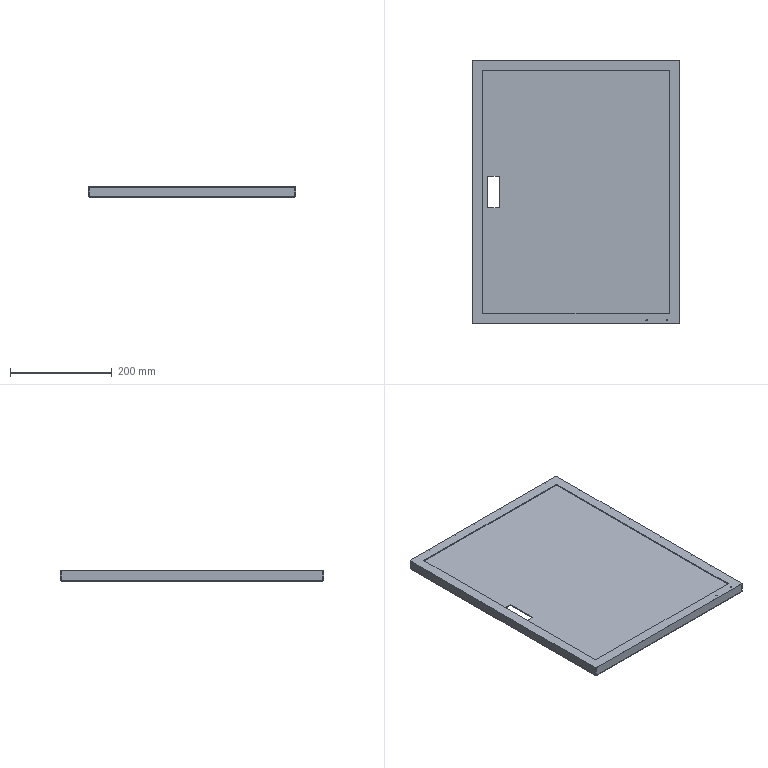Part | STEP file | 11-FG-JX00111 | 1 solid | 36 faces | box 408 x 519 x 20 mm | volume 549034 mm3 | plane 20 | cylinder 12 | sphere 4 | commonest cylinder face diameters 4 x8 2.5 x4
STEP:
#1=CARTESIAN_POINT('',(177.75,-252.5,18.));
#2=VERTEX_POINT('',#1);
#3=CARTESIAN_POINT('',(180.25,-252.5,18.));
#4=VERTEX_POINT('',#3);
#5=CARTESIAN_POINT('',(179.,-252.5,18.));
#6=DIRECTION('',(0.,0.,1.));
#7=DIRECTION('',(1.,0.,0.));
#8=AXIS2_PLACEMENT_3D('',#5,#6,#7);
#9=CIRCLE('',#8,1.25);
#10=EDGE_CURVE('',#2,#4,#9,.T.);
#11=ORIENTED_EDGE('',*,*,#10,.F.);
#12=CARTESIAN_POINT('',(177.75,-252.5,20.));
#13=VERTEX_POINT('',#12);
#14=CARTESIAN_POINT('',(177.75,-252.5,20.));
#15=DIRECTION('',(0.,0.,1.));
#16=VECTOR('',#15,1000.);
#17=LINE('',#14,#16);
#18=EDGE_CURVE('',#2,#13,#17,.T.);
#19=ORIENTED_EDGE('',*,*,#18,.T.);
#20=CARTESIAN_POINT('',(180.25,-252.5,20.));
#21=VERTEX_POINT('',#20);
#22=CARTESIAN_POINT('',(179.,-252.5,20.));
#23=DIRECTION('',(0.,0.,1.));
#24=DIRECTION('',(1.,0.,0.));
#25=AXIS2_PLACEMENT_3D('',#22,#23,#24);
#26=CIRCLE('',#25,1.25);
#27=EDGE_CURVE('',#13,#21,#26,.T.);
#28=ORIENTED_EDGE('',*,*,#27,.T.);
#29=CARTESIAN_POINT('',(180.25,-252.5,20.));
#30=DIRECTION('',(0.,0.,1.));
#31=VECTOR('',#30,1000.);
#32=LINE('',#29,#31);
#33=EDGE_CURVE('',#4,#21,#32,.T.);
#34=ORIENTED_EDGE('',*,*,#33,.F.);
#35=EDGE_LOOP('',(#11,#19,#28,#34));
#36=FACE_OUTER_BOUND('',#35,.T.);
#37=CARTESIAN_POINT('',(179.,-252.5,20.));
#38=DIRECTION('',(0.,0.,1.));
#39=DIRECTION('',(1.,0.,0.));
#40=AXIS2_PLACEMENT_3D('',#37,#38,#39);
#41=CYLINDRICAL_SURFACE('',#40,1.25);
#42=ADVANCED_FACE('',(#36),#41,.F.);
#43=CARTESIAN_POINT('',(137.75,-252.5,18.));
#44=VERTEX_POINT('',#43);
#45=CARTESIAN_POINT('',(140.25,-252.5,18.));
#46=VERTEX_POINT('',#45);
#47=CARTESIAN_POINT('',(139.,-252.5,18.));
#48=DIRECTION('',(0.,0.,1.));
#49=DIRECTION('',(1.,0.,0.));
#50=AXIS2_PLACEMENT_3D('',#47,#48,#49);
#51=CIRCLE('',#50,1.25);
#52=EDGE_CURVE('',#44,#46,#51,.T.);
#53=ORIENTED_EDGE('',*,*,#52,.F.);
#54=CARTESIAN_POINT('',(137.75,-252.5,20.));
#55=VERTEX_POINT('',#54);
#56=CARTESIAN_POINT('',(137.75,-252.5,20.));
#57=DIRECTION('',(0.,0.,1.));
#58=VECTOR('',#57,1000.);
#59=LINE('',#56,#58);
#60=EDGE_CURVE('',#44,#55,#59,.T.);
#61=ORIENTED_EDGE('',*,*,#60,.T.);
#62=CARTESIAN_POINT('',(140.25,-252.5,20.));
#63=VERTEX_POINT('',#62);
#64=CARTESIAN_POINT('',(139.,-252.5,20.));
#65=DIRECTION('',(0.,0.,1.));
#66=DIRECTION('',(1.,0.,0.));
#67=AXIS2_PLACEMENT_3D('',#64,#65,#66);
#68=CIRCLE('',#67,1.25);
#69=EDGE_CURVE('',#55,#63,#68,.T.);
#70=ORIENTED_EDGE('',*,*,#69,.T.);
#71=CARTESIAN_POINT('',(140.25,-252.5,20.));
#72=DIRECTION('',(0.,0.,1.));
#73=VECTOR('',#72,1000.);
#74=LINE('',#71,#73);
#75=EDGE_CURVE('',#46,#63,#74,.T.);
#76=ORIENTED_EDGE('',*,*,#75,.F.);
#77=EDGE_LOOP('',(#53,#61,#70,#76));
#78=FACE_OUTER_BOUND('',#77,.T.);
#79=CARTESIAN_POINT('',(139.,-252.5,20.));
#80=DIRECTION('',(0.,0.,1.));
#81=DIRECTION('',(1.,0.,0.));
#82=AXIS2_PLACEMENT_3D('',#79,#80,#81);
#83=CYLINDRICAL_SURFACE('',#82,1.25);
#84=ADVANCED_FACE('',(#78),#83,.F.);
#85=CARTESIAN_POINT('',(204.,-257.5,2.));
#86=VERTEX_POINT('',#85);
#87=CARTESIAN_POINT('',(204.,257.5,2.));
#88=VERTEX_POINT('',#87);
#89=CARTESIAN_POINT('',(204.,259.5,2.));
#90=DIRECTION('',(0.,1.,0.));
#91=VECTOR('',#90,1000.);
#92=LINE('',#89,#91);
#93=EDGE_CURVE('',#86,#88,#92,.T.);
#94=ORIENTED_EDGE('',*,*,#93,.T.);
#95=CARTESIAN_POINT('',(204.,257.5,20.));
#96=VERTEX_POINT('',#95);
#97=CARTESIAN_POINT('',(204.,257.5,20.));
#98=DIRECTION('',(0.,0.,1.));
#99=VECTOR('',#98,1000.);
#100=LINE('',#97,#99);
#101=EDGE_CURVE('',#88,#96,#100,.T.);
#102=ORIENTED_EDGE('',*,*,#101,.T.);
#103=CARTESIAN_POINT('',(204.,-257.5,20.));
#104=VERTEX_POINT('',#103);
#105=CARTESIAN_POINT('',(204.,259.5,20.));
#106=DIRECTION('',(0.,1.,0.));
#107=VECTOR('',#106,1000.);
#108=LINE('',#105,#107);
#109=EDGE_CURVE('',#104,#96,#108,.T.);
#110=ORIENTED_EDGE('',*,*,#109,.F.);
#111=CARTESIAN_POINT('',(204.,-257.5,20.));
#112=DIRECTION('',(0.,0.,-1.));
#113=VECTOR('',#112,1000.);
#114=LINE('',#111,#113);
#115=EDGE_CURVE('',#104,#86,#114,.T.);
#116=ORIENTED_EDGE('',*,*,#115,.T.);
#117=EDGE_LOOP('',(#94,#102,#110,#116));
#118=FACE_OUTER_BOUND('',#117,.T.);
#119=CARTESIAN_POINT('',(204.,259.5,20.));
#120=DIRECTION('',(-1.,0.,0.));
#121=DIRECTION('',(0.,-1.,0.));
#122=AXIS2_PLACEMENT_3D('',#119,#120,#121);
#123=PLANE('',#122);
#124=ADVANCED_FACE('',(#118),#123,.F.);
#125=CARTESIAN_POINT('',(202.,259.5,2.));
#126=VERTEX_POINT('',#125);
#127=CARTESIAN_POINT('',(-202.,259.5,2.));
#128=VERTEX_POINT('',#127);
#129=CARTESIAN_POINT('',(-204.,259.5,2.));
#130=DIRECTION('',(-1.,0.,0.));
#131=VECTOR('',#130,1000.);
#132=LINE('',#129,#131);
#133=EDGE_CURVE('',#126,#128,#132,.T.);
#134=ORIENTED_EDGE('',*,*,#133,.T.);
#135=CARTESIAN_POINT('',(-202.,259.5,20.));
#136=VERTEX_POINT('',#135);
#137=CARTESIAN_POINT('',(-202.,259.5,20.));
#138=DIRECTION('',(0.,0.,1.));
#139=VECTOR('',#138,1000.);
#140=LINE('',#137,#139);
#141=EDGE_CURVE('',#128,#136,#140,.T.);
#142=ORIENTED_EDGE('',*,*,#141,.T.);
#143=CARTESIAN_POINT('',(202.,259.5,20.));
#144=VERTEX_POINT('',#143);
#145=CARTESIAN_POINT('',(-204.,259.5,20.));
#146=DIRECTION('',(-1.,0.,0.));
#147=VECTOR('',#146,1000.);
#148=LINE('',#145,#147);
#149=EDGE_CURVE('',#144,#136,#148,.T.);
#150=ORIENTED_EDGE('',*,*,#149,.F.);
#151=CARTESIAN_POINT('',(202.,259.5,20.));
#152=DIRECTION('',(0.,0.,-1.));
#153=VECTOR('',#152,1000.);
#154=LINE('',#151,#153);
#155=EDGE_CURVE('',#144,#126,#154,.T.);
#156=ORIENTED_EDGE('',*,*,#155,.T.);
#157=EDGE_LOOP('',(#134,#142,#150,#156));
#158=FACE_OUTER_BOUND('',#157,.T.);
#159=CARTESIAN_POINT('',(-204.,259.5,20.));
#160=DIRECTION('',(0.,-1.,0.));
#161=DIRECTION('',(0.,0.,-1.));
#162=AXIS2_PLACEMENT_3D('',#159,#160,#161);
#163=PLANE('',#162);
#164=ADVANCED_FACE('',(#158),#163,.F.);
#165=CARTESIAN_POINT('',(-204.,257.5,20.));
#166=VERTEX_POINT('',#165);
#167=CARTESIAN_POINT('',(-204.,-257.5,20.));
#168=VERTEX_POINT('',#167);
#169=CARTESIAN_POINT('',(-204.,259.5,20.));
#170=DIRECTION('',(0.,-1.,0.));
#171=VECTOR('',#170,1000.);
#172=LINE('',#169,#171);
#173=EDGE_CURVE('',#166,#168,#172,.T.);
#174=ORIENTED_EDGE('',*,*,#173,.F.);
#175=CARTESIAN_POINT('',(-204.,257.5,2.));
#176=VERTEX_POINT('',#175);
#177=CARTESIAN_POINT('',(-204.,257.5,20.));
#178=DIRECTION('',(0.,0.,-1.));
#179=VECTOR('',#178,1000.);
#180=LINE('',#177,#179);
#181=EDGE_CURVE('',#166,#176,#180,.T.);
#182=ORIENTED_EDGE('',*,*,#181,.T.);
#183=CARTESIAN_POINT('',(-204.,-257.5,2.));
#184=VERTEX_POINT('',#183);
#185=CARTESIAN_POINT('',(-204.,259.5,2.));
#186=DIRECTION('',(0.,-1.,0.));
#187=VECTOR('',#186,1000.);
#188=LINE('',#185,#187);
#189=EDGE_CURVE('',#176,#184,#188,.T.);
#190=ORIENTED_EDGE('',*,*,#189,.T.);
#191=CARTESIAN_POINT('',(-204.,-257.5,20.));
#192=DIRECTION('',(0.,0.,1.));
#193=VECTOR('',#192,1000.);
#194=LINE('',#191,#193);
#195=EDGE_CURVE('',#184,#168,#194,.T.);
#196=ORIENTED_EDGE('',*,*,#195,.T.);
#197=EDGE_LOOP('',(#174,#182,#190,#196));
#198=FACE_OUTER_BOUND('',#197,.T.);
#199=CARTESIAN_POINT('',(-204.,259.5,20.));
#200=DIRECTION('',(1.,0.,0.));
#201=DIRECTION('',(0.,1.,0.));
#202=AXIS2_PLACEMENT_3D('',#199,#200,#201);
#203=PLANE('',#202);
#204=ADVANCED_FACE('',(#198),#203,.F.);
#205=CARTESIAN_POINT('',(-202.,-259.5,2.));
#206=VERTEX_POINT('',#205);
#207=CARTESIAN_POINT('',(202.,-259.5,2.));
#208=VERTEX_POINT('',#207);
#209=CARTESIAN_POINT('',(-204.,-259.5,2.));
#210=DIRECTION('',(1.,0.,0.));
#211=VECTOR('',#210,1000.);
#212=LINE('',#209,#211);
#213=EDGE_CURVE('',#206,#208,#212,.T.);
#214=ORIENTED_EDGE('',*,*,#213,.T.);
#215=CARTESIAN_POINT('',(202.,-259.5,20.));
#216=VERTEX_POINT('',#215);
#217=CARTESIAN_POINT('',(202.,-259.5,20.));
#218=DIRECTION('',(0.,0.,1.));
#219=VECTOR('',#218,1000.);
#220=LINE('',#217,#219);
#221=EDGE_CURVE('',#208,#216,#220,.T.);
#222=ORIENTED_EDGE('',*,*,#221,.T.);
#223=CARTESIAN_POINT('',(-202.,-259.5,20.));
#224=VERTEX_POINT('',#223);
#225=CARTESIAN_POINT('',(-204.,-259.5,20.));
#226=DIRECTION('',(1.,0.,0.));
#227=VECTOR('',#226,1000.);
#228=LINE('',#225,#227);
#229=EDGE_CURVE('',#224,#216,#228,.T.);
#230=ORIENTED_EDGE('',*,*,#229,.F.);
#231=CARTESIAN_POINT('',(-202.,-259.5,20.));
#232=DIRECTION('',(0.,0.,-1.));
#233=VECTOR('',#232,1000.);
#234=LINE('',#231,#233);
#235=EDGE_CURVE('',#224,#206,#234,.T.);
#236=ORIENTED_EDGE('',*,*,#235,.T.);
#237=EDGE_LOOP('',(#214,#222,#230,#236));
#238=FACE_OUTER_BOUND('',#237,.T.);
#239=CARTESIAN_POINT('',(-204.,-259.5,20.));
#240=DIRECTION('',(0.,1.,0.));
#241=DIRECTION('',(0.,0.,1.));
#242=AXIS2_PLACEMENT_3D('',#239,#240,#241);
#243=PLANE('',#242);
#244=ADVANCED_FACE('',(#238),#243,.F.);
#245=CARTESIAN_POINT('',(179.,-252.5,20.));
#246=DIRECTION('',(0.,0.,1.));
#247=DIRECTION('',(1.,0.,0.));
#248=AXIS2_PLACEMENT_3D('',#245,#246,#247);
#249=CIRCLE('',#248,1.25);
#250=EDGE_CURVE('',#21,#13,#249,.T.);
#251=ORIENTED_EDGE('',*,*,#250,.F.);
#252=ORIENTED_EDGE('',*,*,#27,.F.);
#253=EDGE_LOOP('',(#251,#252));
#254=FACE_BOUND('',#253,.T.);
#255=CARTESIAN_POINT('',(139.,-252.5,20.));
#256=DIRECTION('',(0.,0.,1.));
#257=DIRECTION('',(1.,0.,0.));
#258=AXIS2_PLACEMENT_3D('',#255,#256,#257);
#259=CIRCLE('',#258,1.25);
#260=EDGE_CURVE('',#63,#55,#259,.T.);
#261=ORIENTED_EDGE('',*,*,#260,.F.);
#262=ORIENTED_EDGE('',*,*,#69,.F.);
#263=EDGE_LOOP('',(#261,#262));
#264=FACE_BOUND('',#263,.T.);
#265=ORIENTED_EDGE('',*,*,#149,.T.);
#266=CARTESIAN_POINT('',(-202.,257.5,20.));
#267=DIRECTION('',(0.,0.,1.));
#268=DIRECTION('',(1.,0.,0.));
#269=AXIS2_PLACEMENT_3D('',#266,#267,#268);
#270=CIRCLE('',#269,2.);
#271=EDGE_CURVE('',#136,#166,#270,.T.);
#272=ORIENTED_EDGE('',*,*,#271,.T.);
#273=ORIENTED_EDGE('',*,*,#173,.T.);
#274=CARTESIAN_POINT('',(-202.,-257.5,20.));
#275=DIRECTION('',(0.,0.,1.));
#276=DIRECTION('',(1.,0.,0.));
#277=AXIS2_PLACEMENT_3D('',#274,#275,#276);
#278=CIRCLE('',#277,2.);
#279=EDGE_CURVE('',#168,#224,#278,.T.);
#280=ORIENTED_EDGE('',*,*,#279,.T.);
#281=ORIENTED_EDGE('',*,*,#229,.T.);
#282=CARTESIAN_POINT('',(202.,-257.5,20.));
#283=DIRECTION('',(0.,0.,1.));
#284=DIRECTION('',(1.,0.,0.));
#285=AXIS2_PLACEMENT_3D('',#282,#283,#284);
#286=CIRCLE('',#285,2.);
#287=EDGE_CURVE('',#216,#104,#286,.T.);
#288=ORIENTED_EDGE('',*,*,#287,.T.);
#289=ORIENTED_EDGE('',*,*,#109,.T.);
#290=CARTESIAN_POINT('',(202.,257.5,20.));
#291=DIRECTION('',(0.,0.,1.));
#292=DIRECTION('',(1.,0.,0.));
#293=AXIS2_PLACEMENT_3D('',#290,#291,#292);
#294=CIRCLE('',#293,2.);
#295=EDGE_CURVE('',#96,#144,#294,.T.);
#296=ORIENTED_EDGE('',*,*,#295,.T.);
#297=EDGE_LOOP('',(#265,#272,#273,#280,#281,#288,#289,#296));
#298=FACE_OUTER_BOUND('',#297,.T.);
#299=CARTESIAN_POINT('',(-184.,239.5,20.));
#300=VERTEX_POINT('',#299);
#301=CARTESIAN_POINT('',(-184.,-239.5,20.));
#302=VERTEX_POINT('',#301);
#303=CARTESIAN_POINT('',(-184.,257.5,20.));
#304=DIRECTION('',(0.,-1.,0.));
#305=VECTOR('',#304,1000.);
#306=LINE('',#303,#305);
#307=EDGE_CURVE('',#300,#302,#306,.T.);
#308=ORIENTED_EDGE('',*,*,#307,.F.);
#309=CARTESIAN_POINT('',(184.,239.5,20.));
#310=VERTEX_POINT('',#309);
#311=CARTESIAN_POINT('',(-202.,239.5,20.));
#312=DIRECTION('',(-1.,0.,0.));
#313=VECTOR('',#312,1000.);
#314=LINE('',#311,#313);
#315=EDGE_CURVE('',#310,#300,#314,.T.);
#316=ORIENTED_EDGE('',*,*,#315,.F.);
#317=CARTESIAN_POINT('',(184.,-239.5,20.));
#318=VERTEX_POINT('',#317);
#319=CARTESIAN_POINT('',(184.,257.5,20.));
#320=DIRECTION('',(0.,1.,0.));
#321=VECTOR('',#320,1000.);
#322=LINE('',#319,#321);
#323=EDGE_CURVE('',#318,#310,#322,.T.);
#324=ORIENTED_EDGE('',*,*,#323,.F.);
#325=CARTESIAN_POINT('',(-202.,-239.5,20.));
#326=DIRECTION('',(1.,0.,0.));
#327=VECTOR('',#326,1000.);
#328=LINE('',#325,#327);
#329=EDGE_CURVE('',#302,#318,#328,.T.);
#330=ORIENTED_EDGE('',*,*,#329,.F.);
#331=EDGE_LOOP('',(#308,#316,#324,#330));
#332=FACE_BOUND('',#331,.T.);
#333=CARTESIAN_POINT('',(0.,0.,20.));
#334=DIRECTION('',(0.,0.,1.));
#335=DIRECTION('',(1.,0.,0.));
#336=AXIS2_PLACEMENT_3D('',#333,#334,#335);
#337=PLANE('',#336);
#338=ADVANCED_FACE('',(#254,#264,#298,#332),#337,.T.);
#339=CARTESIAN_POINT('',(-202.,-257.5,0.));
#340=VERTEX_POINT('',#339);
#341=CARTESIAN_POINT('',(-202.,257.5,0.));
#342=VERTEX_POINT('',#341);
#343=CARTESIAN_POINT('',(-202.,0.,0.));
#344=DIRECTION('',(0.,1.,0.));
#345=VECTOR('',#344,1000.);
#346=LINE('',#343,#345);
#347=EDGE_CURVE('',#340,#342,#346,.T.);
#348=ORIENTED_EDGE('',*,*,#347,.T.);
#349=CARTESIAN_POINT('',(202.,257.5,0.));
#350=VERTEX_POINT('',#349);
#351=CARTESIAN_POINT('',(0.,257.5,0.));
#352=DIRECTION('',(1.,0.,0.));
#353=VECTOR('',#352,1000.);
#354=LINE('',#351,#353);
#355=EDGE_CURVE('',#342,#350,#354,.T.);
#356=ORIENTED_EDGE('',*,*,#355,.T.);
#357=CARTESIAN_POINT('',(202.,-257.5,0.));
#358=VERTEX_POINT('',#357);
#359=CARTESIAN_POINT('',(202.,0.,0.));
#360=DIRECTION('',(0.,-1.,0.));
#361=VECTOR('',#360,1000.);
#362=LINE('',#359,#361);
#363=EDGE_CURVE('',#350,#358,#362,.T.);
#364=ORIENTED_EDGE('',*,*,#363,.T.);
#365=CARTESIAN_POINT('',(0.,-257.5,0.));
#366=DIRECTION('',(-1.,0.,0.));
#367=VECTOR('',#366,1000.);
#368=LINE('',#365,#367);
#369=EDGE_CURVE('',#358,#340,#368,.T.);
#370=ORIENTED_EDGE('',*,*,#369,.T.);
#371=EDGE_LOOP('',(#348,#356,#364,#370));
#372=FACE_OUTER_BOUND('',#371,.T.);
#373=CARTESIAN_POINT('',(-174.,-31.,0.));
#374=VERTEX_POINT('',#373);
#375=CARTESIAN_POINT('',(-151.2,-31.,0.));
#376=VERTEX_POINT('',#375);
#377=CARTESIAN_POINT('',(-151.2,-31.,0.));
#378=DIRECTION('',(1.,0.,0.));
#379=VECTOR('',#378,1000.);
#380=LINE('',#377,#379);
#381=EDGE_CURVE('',#374,#376,#380,.T.);
#382=ORIENTED_EDGE('',*,*,#381,.T.);
#383=CARTESIAN_POINT('',(-151.2,31.,0.));
#384=VERTEX_POINT('',#383);
#385=CARTESIAN_POINT('',(-151.2,31.,0.));
#386=DIRECTION('',(0.,1.,0.));
#387=VECTOR('',#386,1000.);
#388=LINE('',#385,#387);
#389=EDGE_CURVE('',#376,#384,#388,.T.);
#390=ORIENTED_EDGE('',*,*,#389,.T.);
#391=CARTESIAN_POINT('',(-174.,31.,0.));
#392=VERTEX_POINT('',#391);
#393=CARTESIAN_POINT('',(-151.2,31.,0.));
#394=DIRECTION('',(-1.,0.,0.));
#395=VECTOR('',#394,1000.);
#396=LINE('',#393,#395);
#397=EDGE_CURVE('',#384,#392,#396,.T.);
#398=ORIENTED_EDGE('',*,*,#397,.T.);
#399=CARTESIAN_POINT('',(-174.,31.,0.));
#400=DIRECTION('',(0.,-1.,0.));
#401=VECTOR('',#400,1000.);
#402=LINE('',#399,#401);
#403=EDGE_CURVE('',#392,#374,#402,.T.);
#404=ORIENTED_EDGE('',*,*,#403,.T.);
#405=EDGE_LOOP('',(#382,#390,#398,#404));
#406=FACE_BOUND('',#405,.T.);
#407=CARTESIAN_POINT('',(0.,0.,0.));
#408=DIRECTION('',(0.,0.,1.));
#409=DIRECTION('',(1.,0.,0.));
#410=AXIS2_PLACEMENT_3D('',#407,#408,#409);
#411=PLANE('',#410);
#412=ADVANCED_FACE('',(#372,#406),#411,.F.);
#413=CARTESIAN_POINT('',(179.,-252.5,18.));
#414=DIRECTION('',(0.,0.,1.));
#415=DIRECTION('',(1.,0.,0.));
#416=AXIS2_PLACEMENT_3D('',#413,#414,#415);
#417=CIRCLE('',#416,1.25);
#418=EDGE_CURVE('',#4,#2,#417,.T.);
#419=ORIENTED_EDGE('',*,*,#418,.T.);
#420=ORIENTED_EDGE('',*,*,#10,.T.);
#421=EDGE_LOOP('',(#419,#420));
#422=FACE_BOUND('',#421,.T.);
#423=CARTESIAN_POINT('',(139.,-252.5,18.));
#424=DIRECTION('',(0.,0.,1.));
#425=DIRECTION('',(1.,0.,0.));
#426=AXIS2_PLACEMENT_3D('',#423,#424,#425);
#427=CIRCLE('',#426,1.25);
#428=EDGE_CURVE('',#46,#44,#427,.T.);
#429=ORIENTED_EDGE('',*,*,#428,.T.);
#430=ORIENTED_EDGE('',*,*,#52,.T.);
#431=EDGE_LOOP('',(#429,#430));
#432=FACE_BOUND('',#431,.T.);
#433=CARTESIAN_POINT('',(184.,239.5,18.));
#434=VERTEX_POINT('',#433);
#435=CARTESIAN_POINT('',(-184.,239.5,18.));
#436=VERTEX_POINT('',#435);
#437=CARTESIAN_POINT('',(-202.,239.5,18.));
#438=DIRECTION('',(-1.,0.,0.));
#439=VECTOR('',#438,1000.);
#440=LINE('',#437,#439);
#441=EDGE_CURVE('',#434,#436,#440,.T.);
#442=ORIENTED_EDGE('',*,*,#441,.T.);
#443=CARTESIAN_POINT('',(-184.,-239.5,18.));
#444=VERTEX_POINT('',#443);
#445=CARTESIAN_POINT('',(-184.,257.5,18.));
#446=DIRECTION('',(0.,-1.,0.));
#447=VECTOR('',#446,1000.);
#448=LINE('',#445,#447);
#449=EDGE_CURVE('',#436,#444,#448,.T.);
#450=ORIENTED_EDGE('',*,*,#449,.T.);
#451=CARTESIAN_POINT('',(184.,-239.5,18.));
#452=VERTEX_POINT('',#451);
#453=CARTESIAN_POINT('',(-202.,-239.5,18.));
#454=DIRECTION('',(1.,0.,0.));
#455=VECTOR('',#454,1000.);
#456=LINE('',#453,#455);
#457=EDGE_CURVE('',#444,#452,#456,.T.);
#458=ORIENTED_EDGE('',*,*,#457,.T.);
#459=CARTESIAN_POINT('',(184.,257.5,18.));
#460=DIRECTION('',(0.,1.,0.));
#461=VECTOR('',#460,1000.);
#462=LINE('',#459,#461);
#463=EDGE_CURVE('',#452,#434,#462,.T.);
#464=ORIENTED_EDGE('',*,*,#463,.T.);
#465=EDGE_LOOP('',(#442,#450,#458,#464));
#466=FACE_BOUND('',#465,.T.);
#467=CARTESIAN_POINT('',(-202.,257.5,18.));
#468=VERTEX_POINT('',#467);
#469=CARTESIAN_POINT('',(-202.,-257.5,18.));
#470=VERTEX_POINT('',#469);
#471=CARTESIAN_POINT('',(-202.,257.5,18.));
#472=DIRECTION('',(0.,-1.,0.));
#473=VECTOR('',#472,1000.);
#474=LINE('',#471,#473);
#475=EDGE_CURVE('',#468,#470,#474,.T.);
#476=ORIENTED_EDGE('',*,*,#475,.F.);
#477=CARTESIAN_POINT('',(202.,257.5,18.));
#478=VERTEX_POINT('',#477);
#479=CARTESIAN_POINT('',(-202.,257.5,18.));
#480=DIRECTION('',(-1.,0.,0.));
#481=VECTOR('',#480,1000.);
#482=LINE('',#479,#481);
#483=EDGE_CURVE('',#478,#468,#482,.T.);
#484=ORIENTED_EDGE('',*,*,#483,.F.);
#485=CARTESIAN_POINT('',(202.,-257.5,18.));
#486=VERTEX_POINT('',#485);
#487=CARTESIAN_POINT('',(202.,257.5,18.));
#488=DIRECTION('',(0.,1.,0.));
#489=VECTOR('',#488,1000.);
#490=LINE('',#487,#489);
#491=EDGE_CURVE('',#486,#478,#490,.T.);
#492=ORIENTED_EDGE('',*,*,#491,.F.);
#493=CARTESIAN_POINT('',(-202.,-257.5,18.));
#494=DIRECTION('',(1.,0.,0.));
#495=VECTOR('',#494,1000.);
#496=LINE('',#493,#495);
#497=EDGE_CURVE('',#470,#486,#496,.T.);
#498=ORIENTED_EDGE('',*,*,#497,.F.);
#499=EDGE_LOOP('',(#476,#484,#492,#498));
#500=FACE_OUTER_BOUND('',#499,.T.);
#501=CARTESIAN_POINT('',(0.,0.,18.));
#502=DIRECTION('',(0.,0.,1.));
#503=DIRECTION('',(1.,0.,0.));
#504=AXIS2_PLACEMENT_3D('',#501,#502,#503);
#505=PLANE('',#504);
#506=ADVANCED_FACE('',(#422,#432,#466,#500),#505,.F.);
#507=ORIENTED_EDGE('',*,*,#307,.T.);
#508=CARTESIAN_POINT('',(-184.,-239.5,18.));
#509=DIRECTION('',(0.,0.,1.));
#510=VECTOR('',#509,1000.);
#511=LINE('',#508,#510);
#512=EDGE_CURVE('',#444,#302,#511,.T.);
#513=ORIENTED_EDGE('',*,*,#512,.F.);
#514=ORIENTED_EDGE('',*,*,#449,.F.);
#515=CARTESIAN_POINT('',(-184.,239.5,18.));
#516=DIRECTION('',(0.,0.,1.));
#517=VECTOR('',#516,1000.);
#518=LINE('',#515,#517);
#519=EDGE_CURVE('',#436,#300,#518,.T.);
#520=ORIENTED_EDGE('',*,*,#519,.T.);
#521=EDGE_LOOP('',(#507,#513,#514,#520));
#522=FACE_OUTER_BOUND('',#521,.T.);
#523=CARTESIAN_POINT('',(-184.,257.5,18.));
#524=DIRECTION('',(-1.,0.,0.));
#525=DIRECTION('',(0.,-1.,0.));
#526=AXIS2_PLACEMENT_3D('',#523,#524,#525);
#527=PLANE('',#526);
#528=ADVANCED_FACE('',(#522),#527,.F.);
#529=ORIENTED_EDGE('',*,*,#315,.T.);
#530=ORIENTED_EDGE('',*,*,#519,.F.);
#531=ORIENTED_EDGE('',*,*,#441,.F.);
#532=CARTESIAN_POINT('',(184.,239.5,18.));
#533=DIRECTION('',(0.,0.,1.));
#534=VECTOR('',#533,1000.);
#535=LINE('',#532,#534);
#536=EDGE_CURVE('',#434,#310,#535,.T.);
#537=ORIENTED_EDGE('',*,*,#536,.T.);
#538=EDGE_LOOP('',(#529,#530,#531,#537));
#539=FACE_OUTER_BOUND('',#538,.T.);
#540=CARTESIAN_POINT('',(-202.,239.5,18.));
#541=DIRECTION('',(0.,1.,0.));
#542=DIRECTION('',(0.,0.,1.));
#543=AXIS2_PLACEMENT_3D('',#540,#541,#542);
#544=PLANE('',#543);
#545=ADVANCED_FACE('',(#539),#544,.F.);
#546=ORIENTED_EDGE('',*,*,#323,.T.);
#547=ORIENTED_EDGE('',*,*,#536,.F.);
#548=ORIENTED_EDGE('',*,*,#463,.F.);
#549=CARTESIAN_POINT('',(184.,-239.5,18.));
#550=DIRECTION('',(0.,0.,1.));
#551=VECTOR('',#550,1000.);
#552=LINE('',#549,#551);
#553=EDGE_CURVE('',#452,#318,#552,.T.);
#554=ORIENTED_EDGE('',*,*,#553,.T.);
#555=EDGE_LOOP('',(#546,#547,#548,#554));
#556=FACE_OUTER_BOUND('',#555,.T.);
#557=CARTESIAN_POINT('',(184.,257.5,18.));
#558=DIRECTION('',(1.,0.,0.));
#559=DIRECTION('',(0.,1.,0.));
#560=AXIS2_PLACEMENT_3D('',#557,#558,#559);
#561=PLANE('',#560);
#562=ADVANCED_FACE('',(#556),#561,.F.);
#563=ORIENTED_EDGE('',*,*,#329,.T.);
#564=ORIENTED_EDGE('',*,*,#553,.F.);
#565=ORIENTED_EDGE('',*,*,#457,.F.);
#566=ORIENTED_EDGE('',*,*,#512,.T.);
#567=EDGE_LOOP('',(#563,#564,#565,#566));
#568=FACE_OUTER_BOUND('',#567,.T.);
#569=CARTESIAN_POINT('',(-202.,-239.5,18.));
#570=DIRECTION('',(0.,-1.,0.));
#571=DIRECTION('',(0.,0.,-1.));
#572=AXIS2_PLACEMENT_3D('',#569,#570,#571);
#573=PLANE('',#572);
#574=ADVANCED_FACE('',(#568),#573,.F.);
#575=CARTESIAN_POINT('',(-151.2,-31.,2.));
#576=VERTEX_POINT('',#575);
#577=CARTESIAN_POINT('',(-151.2,31.,2.));
#578=VERTEX_POINT('',#577);
#579=CARTESIAN_POINT('',(-151.2,31.,2.));
#580=DIRECTION('',(0.,1.,0.));
#581=VECTOR('',#580,1000.);
#582=LINE('',#579,#581);
#583=EDGE_CURVE('',#576,#578,#582,.T.);
#584=ORIENTED_EDGE('',*,*,#583,.F.);
#585=CARTESIAN_POINT('',(-174.,-31.,2.));
#586=VERTEX_POINT('',#585);
#587=CARTESIAN_POINT('',(-151.2,-31.,2.));
#588=DIRECTION('',(1.,0.,0.));
#589=VECTOR('',#588,1000.);
#590=LINE('',#587,#589);
#591=EDGE_CURVE('',#586,#576,#590,.T.);
#592=ORIENTED_EDGE('',*,*,#591,.F.);
#593=CARTESIAN_POINT('',(-174.,31.,2.));
#594=VERTEX_POINT('',#593);
#595=CARTESIAN_POINT('',(-174.,31.,2.));
#596=DIRECTION('',(0.,-1.,0.));
#597=VECTOR('',#596,1000.);
#598=LINE('',#595,#597);
#599=EDGE_CURVE('',#594,#586,#598,.T.);
#600=ORIENTED_EDGE('',*,*,#599,.F.);
#601=CARTESIAN_POINT('',(-151.2,31.,2.));
#602=DIRECTION('',(-1.,0.,0.));
#603=VECTOR('',#602,1000.);
#604=LINE('',#601,#603);
#605=EDGE_CURVE('',#578,#594,#604,.T.);
#606=ORIENTED_EDGE('',*,*,#605,.F.);
#607=EDGE_LOOP('',(#584,#592,#600,#606));
#608=FACE_BOUND('',#607,.T.);
#609=CARTESIAN_POINT('',(202.,-257.5,2.));
#610=VERTEX_POINT('',#609);
#611=CARTESIAN_POINT('',(202.,257.5,2.));
#612=VERTEX_POINT('',#611);
#613=CARTESIAN_POINT('',(202.,259.5,2.));
#614=DIRECTION('',(0.,1.,0.));
#615=VECTOR('',#614,1000.);
#616=LINE('',#613,#615);
#617=EDGE_CURVE('',#610,#612,#616,.T.);
#618=ORIENTED_EDGE('',*,*,#617,.T.);
#619=CARTESIAN_POINT('',(-202.,257.5,2.));
#620=VERTEX_POINT('',#619);
#621=CARTESIAN_POINT('',(-204.,257.5,2.));
#622=DIRECTION('',(-1.,0.,0.));
#623=VECTOR('',#622,1000.);
#624=LINE('',#621,#623);
#625=EDGE_CURVE('',#612,#620,#624,.T.);
#626=ORIENTED_EDGE('',*,*,#625,.T.);
#627=CARTESIAN_POINT('',(-202.,-257.5,2.));
#628=VERTEX_POINT('',#627);
#629=CARTESIAN_POINT('',(-202.,259.5,2.));
#630=DIRECTION('',(0.,-1.,0.));
#631=VECTOR('',#630,1000.);
#632=LINE('',#629,#631);
#633=EDGE_CURVE('',#620,#628,#632,.T.);
#634=ORIENTED_EDGE('',*,*,#633,.T.);
#635=CARTESIAN_POINT('',(-204.,-257.5,2.));
#636=DIRECTION('',(1.,0.,0.));
#637=VECTOR('',#636,1000.);
#638=LINE('',#635,#637);
#639=EDGE_CURVE('',#628,#610,#638,.T.);
#640=ORIENTED_EDGE('',*,*,#639,.T.);
#641=EDGE_LOOP('',(#618,#626,#634,#640));
#642=FACE_OUTER_BOUND('',#641,.T.);
#643=CARTESIAN_POINT('',(0.,0.,2.));
#644=DIRECTION('',(0.,0.,1.));
#645=DIRECTION('',(1.,0.,0.));
#646=AXIS2_PLACEMENT_3D('',#643,#644,#645);
#647=PLANE('',#646);
#648=ADVANCED_FACE('',(#608,#642),#647,.T.);
#649=CARTESIAN_POINT('',(-202.,-257.5,20.));
#650=DIRECTION('',(0.,0.,-1.));
#651=VECTOR('',#650,1000.);
#652=LINE('',#649,#651);
#653=EDGE_CURVE('',#470,#628,#652,.T.);
#654=ORIENTED_EDGE('',*,*,#653,.F.);
#655=ORIENTED_EDGE('',*,*,#497,.T.);
#656=CARTESIAN_POINT('',(202.,-257.5,20.));
#657=DIRECTION('',(0.,0.,-1.));
#658=VECTOR('',#657,1000.);
#659=LINE('',#656,#658);
#660=EDGE_CURVE('',#486,#610,#659,.T.);
#661=ORIENTED_EDGE('',*,*,#660,.T.);
#662=ORIENTED_EDGE('',*,*,#639,.F.);
#663=EDGE_LOOP('',(#654,#655,#661,#662));
#664=FACE_OUTER_BOUND('',#663,.T.);
#665=CARTESIAN_POINT('',(-204.,-257.5,20.));
#666=DIRECTION('',(0.,1.,0.));
#667=DIRECTION('',(0.,0.,1.));
#668=AXIS2_PLACEMENT_3D('',#665,#666,#667);
#669=PLANE('',#668);
#670=ADVANCED_FACE('',(#664),#669,.T.);
#671=CARTESIAN_POINT('',(-202.,257.5,20.));
#672=DIRECTION('',(0.,0.,-1.));
#673=VECTOR('',#672,1000.);
#674=LINE('',#671,#673);
#675=EDGE_CURVE('',#468,#620,#674,.T.);
#676=ORIENTED_EDGE('',*,*,#675,.F.);
#677=ORIENTED_EDGE('',*,*,#475,.T.);
#678=ORIENTED_EDGE('',*,*,#653,.T.);
#679=ORIENTED_EDGE('',*,*,#633,.F.);
#680=EDGE_LOOP('',(#676,#677,#678,#679));
#681=FACE_OUTER_BOUND('',#680,.T.);
#682=CARTESIAN_POINT('',(-202.,259.5,20.));
#683=DIRECTION('',(1.,0.,0.));
#684=DIRECTION('',(0.,1.,0.));
#685=AXIS2_PLACEMENT_3D('',#682,#683,#684);
#686=PLANE('',#685);
#687=ADVANCED_FACE('',(#681),#686,.T.);
#688=CARTESIAN_POINT('',(202.,257.5,20.));
#689=DIRECTION('',(0.,0.,-1.));
#690=VECTOR('',#689,1000.);
#691=LINE('',#688,#690);
#692=EDGE_CURVE('',#478,#612,#691,.T.);
#693=ORIENTED_EDGE('',*,*,#692,.F.);
#694=ORIENTED_EDGE('',*,*,#483,.T.);
#695=ORIENTED_EDGE('',*,*,#675,.T.);
#696=ORIENTED_EDGE('',*,*,#625,.F.);
#697=EDGE_LOOP('',(#693,#694,#695,#696));
#698=FACE_OUTER_BOUND('',#697,.T.);
#699=CARTESIAN_POINT('',(-204.,257.5,20.));
#700=DIRECTION('',(0.,-1.,0.));
#701=DIRECTION('',(0.,0.,-1.));
#702=AXIS2_PLACEMENT_3D('',#699,#700,#701);
#703=PLANE('',#702);
#704=ADVANCED_FACE('',(#698),#703,.T.);
#705=ORIENTED_EDGE('',*,*,#660,.F.);
#706=ORIENTED_EDGE('',*,*,#491,.T.);
#707=ORIENTED_EDGE('',*,*,#692,.T.);
#708=ORIENTED_EDGE('',*,*,#617,.F.);
#709=EDGE_LOOP('',(#705,#706,#707,#708));
#710=FACE_OUTER_BOUND('',#709,.T.);
#711=CARTESIAN_POINT('',(202.,259.5,20.));
#712=DIRECTION('',(-1.,0.,0.));
#713=DIRECTION('',(0.,-1.,0.));
#714=AXIS2_PLACEMENT_3D('',#711,#712,#713);
#715=PLANE('',#714);
#716=ADVANCED_FACE('',(#710),#715,.T.);
#717=ORIENTED_EDGE('',*,*,#583,.T.);
#718=CARTESIAN_POINT('',(-151.2,31.,0.));
#719=DIRECTION('',(0.,0.,1.));
#720=VECTOR('',#719,1000.);
#721=LINE('',#718,#720);
#722=EDGE_CURVE('',#384,#578,#721,.T.);
#723=ORIENTED_EDGE('',*,*,#722,.F.);
#724=ORIENTED_EDGE('',*,*,#389,.F.);
#725=CARTESIAN_POINT('',(-151.2,-31.,0.));
#726=DIRECTION('',(0.,0.,1.));
#727=VECTOR('',#726,1000.);
#728=LINE('',#725,#727);
#729=EDGE_CURVE('',#376,#576,#728,.T.);
#730=ORIENTED_EDGE('',*,*,#729,.T.);
#731=EDGE_LOOP('',(#717,#723,#724,#730));
#732=FACE_OUTER_BOUND('',#731,.T.);
#733=CARTESIAN_POINT('',(-151.2,31.,0.));
#734=DIRECTION('',(1.,0.,0.));
#735=DIRECTION('',(0.,1.,0.));
#736=AXIS2_PLACEMENT_3D('',#733,#734,#735);
#737=PLANE('',#736);
#738=ADVANCED_FACE('',(#732),#737,.F.);
#739=ORIENTED_EDGE('',*,*,#591,.T.);
#740=ORIENTED_EDGE('',*,*,#729,.F.);
#741=ORIENTED_EDGE('',*,*,#381,.F.);
#742=CARTESIAN_POINT('',(-174.,-31.,0.));
#743=DIRECTION('',(0.,0.,1.));
#744=VECTOR('',#743,1000.);
#745=LINE('',#742,#744);
#746=EDGE_CURVE('',#374,#586,#745,.T.);
#747=ORIENTED_EDGE('',*,*,#746,.T.);
#748=EDGE_LOOP('',(#739,#740,#741,#747));
#749=FACE_OUTER_BOUND('',#748,.T.);
#750=CARTESIAN_POINT('',(-151.2,-31.,0.));
#751=DIRECTION('',(0.,-1.,0.));
#752=DIRECTION('',(1.,0.,0.));
#753=AXIS2_PLACEMENT_3D('',#750,#751,#752);
#754=PLANE('',#753);
#755=ADVANCED_FACE('',(#749),#754,.F.);
#756=ORIENTED_EDGE('',*,*,#599,.T.);
#757=ORIENTED_EDGE('',*,*,#746,.F.);
#758=ORIENTED_EDGE('',*,*,#403,.F.);
#759=CARTESIAN_POINT('',(-174.,31.,0.));
#760=DIRECTION('',(0.,0.,1.));
#761=VECTOR('',#760,1000.);
#762=LINE('',#759,#761);
#763=EDGE_CURVE('',#392,#594,#762,.T.);
#764=ORIENTED_EDGE('',*,*,#763,.T.);
#765=EDGE_LOOP('',(#756,#757,#758,#764));
#766=FACE_OUTER_BOUND('',#765,.T.);
#767=CARTESIAN_POINT('',(-174.,31.,0.));
#768=DIRECTION('',(-1.,0.,0.));
#769=DIRECTION('',(0.,-1.,0.));
#770=AXIS2_PLACEMENT_3D('',#767,#768,#769);
#771=PLANE('',#770);
#772=ADVANCED_FACE('',(#766),#771,.F.);
#773=ORIENTED_EDGE('',*,*,#605,.T.);
#774=ORIENTED_EDGE('',*,*,#763,.F.);
#775=ORIENTED_EDGE('',*,*,#397,.F.);
#776=ORIENTED_EDGE('',*,*,#722,.T.);
#777=EDGE_LOOP('',(#773,#774,#775,#776));
#778=FACE_OUTER_BOUND('',#777,.T.);
#779=CARTESIAN_POINT('',(-151.2,31.,0.));
#780=DIRECTION('',(0.,1.,0.));
#781=DIRECTION('',(-1.,0.,0.));
#782=AXIS2_PLACEMENT_3D('',#779,#780,#781);
#783=PLANE('',#782);
#784=ADVANCED_FACE('',(#778),#783,.F.);
#785=ORIENTED_EDGE('',*,*,#287,.F.);
#786=ORIENTED_EDGE('',*,*,#221,.F.);
#787=CARTESIAN_POINT('',(202.,-257.5,2.));
#788=DIRECTION('',(0.,0.,-1.));
#789=DIRECTION('',(-1.,0.,0.));
#790=AXIS2_PLACEMENT_3D('',#787,#788,#789);
#791=CIRCLE('',#790,2.);
#792=EDGE_CURVE('',#86,#208,#791,.T.);
#793=ORIENTED_EDGE('',*,*,#792,.F.);
#794=ORIENTED_EDGE('',*,*,#115,.F.);
#795=EDGE_LOOP('',(#785,#786,#793,#794));
#796=FACE_OUTER_BOUND('',#795,.T.);
#797=CARTESIAN_POINT('',(202.,-257.5,20.));
#798=DIRECTION('',(0.,0.,-1.));
#799=DIRECTION('',(-1.,0.,0.));
#800=AXIS2_PLACEMENT_3D('',#797,#798,#799);
#801=CYLINDRICAL_SURFACE('',#800,2.);
#802=ADVANCED_FACE('',(#796),#801,.T.);
#803=ORIENTED_EDGE('',*,*,#279,.F.);
#804=ORIENTED_EDGE('',*,*,#195,.F.);
#805=CARTESIAN_POINT('',(-202.,-257.5,2.));
#806=DIRECTION('',(0.,0.,-1.));
#807=DIRECTION('',(-1.,0.,0.));
#808=AXIS2_PLACEMENT_3D('',#805,#806,#807);
#809=CIRCLE('',#808,2.);
#810=EDGE_CURVE('',#206,#184,#809,.T.);
#811=ORIENTED_EDGE('',*,*,#810,.F.);
#812=ORIENTED_EDGE('',*,*,#235,.F.);
#813=EDGE_LOOP('',(#803,#804,#811,#812));
#814=FACE_OUTER_BOUND('',#813,.T.);
#815=CARTESIAN_POINT('',(-202.,-257.5,20.));
#816=DIRECTION('',(0.,0.,-1.));
#817=DIRECTION('',(-1.,0.,0.));
#818=AXIS2_PLACEMENT_3D('',#815,#816,#817);
#819=CYLINDRICAL_SURFACE('',#818,2.);
#820=ADVANCED_FACE('',(#814),#819,.T.);
#821=CARTESIAN_POINT('',(202.,-257.5,2.));
#822=DIRECTION('',(1.,0.,0.));
#823=DIRECTION('',(0.,0.,-1.));
#824=AXIS2_PLACEMENT_3D('',#821,#822,#823);
#825=CIRCLE('',#824,2.);
#826=EDGE_CURVE('',#208,#358,#825,.T.);
#827=ORIENTED_EDGE('',*,*,#826,.F.);
#828=ORIENTED_EDGE('',*,*,#213,.F.);
#829=CARTESIAN_POINT('',(-202.,-257.5,2.));
#830=DIRECTION('',(-1.,0.,0.));
#831=DIRECTION('',(0.,0.,1.));
#832=AXIS2_PLACEMENT_3D('',#829,#830,#831);
#833=CIRCLE('',#832,2.);
#834=EDGE_CURVE('',#340,#206,#833,.T.);
#835=ORIENTED_EDGE('',*,*,#834,.F.);
#836=ORIENTED_EDGE('',*,*,#369,.F.);
#837=EDGE_LOOP('',(#827,#828,#835,#836));
#838=FACE_OUTER_BOUND('',#837,.T.);
#839=CARTESIAN_POINT('',(-204.,-257.5,2.));
#840=DIRECTION('',(1.,0.,0.));
#841=DIRECTION('',(0.,0.,-1.));
#842=AXIS2_PLACEMENT_3D('',#839,#840,#841);
#843=CYLINDRICAL_SURFACE('',#842,2.);
#844=ADVANCED_FACE('',(#838),#843,.T.);
#845=ORIENTED_EDGE('',*,*,#792,.T.);
#846=ORIENTED_EDGE('',*,*,#826,.T.);
#847=CARTESIAN_POINT('',(202.,-257.5,2.));
#848=DIRECTION('',(0.,1.,0.));
#849=DIRECTION('',(0.,0.,-1.));
#850=AXIS2_PLACEMENT_3D('',#847,#848,#849);
#851=CIRCLE('',#850,2.);
#852=EDGE_CURVE('',#86,#358,#851,.T.);
#853=ORIENTED_EDGE('',*,*,#852,.F.);
#854=EDGE_LOOP('',(#845,#846,#853));
#855=FACE_OUTER_BOUND('',#854,.T.);
#856=CARTESIAN_POINT('',(202.,-257.5,2.));
#857=DIRECTION('',(0.,1.,0.));
#858=DIRECTION('',(1.,0.,0.));
#859=AXIS2_PLACEMENT_3D('',#856,#857,#858);
#860=SPHERICAL_SURFACE('',#859,2.);
#861=ADVANCED_FACE('',(#855),#860,.T.);
#862=ORIENTED_EDGE('',*,*,#834,.T.);
#863=ORIENTED_EDGE('',*,*,#810,.T.);
#864=CARTESIAN_POINT('',(-202.,-257.5,2.));
#865=DIRECTION('',(0.,1.,0.));
#866=DIRECTION('',(0.,0.,-1.));
#867=AXIS2_PLACEMENT_3D('',#864,#865,#866);
#868=CIRCLE('',#867,2.);
#869=EDGE_CURVE('',#340,#184,#868,.T.);
#870=ORIENTED_EDGE('',*,*,#869,.F.);
#871=EDGE_LOOP('',(#862,#863,#870));
#872=FACE_OUTER_BOUND('',#871,.T.);
#873=CARTESIAN_POINT('',(-202.,-257.5,2.));
#874=DIRECTION('',(0.,1.,0.));
#875=DIRECTION('',(1.,0.,0.));
#876=AXIS2_PLACEMENT_3D('',#873,#874,#875);
#877=SPHERICAL_SURFACE('',#876,2.);
#878=ADVANCED_FACE('',(#872),#877,.T.);
#879=ORIENTED_EDGE('',*,*,#852,.T.);
#880=ORIENTED_EDGE('',*,*,#363,.F.);
#881=CARTESIAN_POINT('',(202.,257.5,2.));
#882=DIRECTION('',(0.,1.,0.));
#883=DIRECTION('',(0.,0.,1.));
#884=AXIS2_PLACEMENT_3D('',#881,#882,#883);
#885=CIRCLE('',#884,2.);
#886=EDGE_CURVE('',#88,#350,#885,.T.);
#887=ORIENTED_EDGE('',*,*,#886,.F.);
#888=ORIENTED_EDGE('',*,*,#93,.F.);
#889=EDGE_LOOP('',(#879,#880,#887,#888));
#890=FACE_OUTER_BOUND('',#889,.T.);
#891=CARTESIAN_POINT('',(202.,259.5,2.));
#892=DIRECTION('',(0.,1.,0.));
#893=DIRECTION('',(-1.,0.,0.));
#894=AXIS2_PLACEMENT_3D('',#891,#892,#893);
#895=CYLINDRICAL_SURFACE('',#894,2.);
#896=ADVANCED_FACE('',(#890),#895,.T.);
#897=ORIENTED_EDGE('',*,*,#295,.F.);
#898=ORIENTED_EDGE('',*,*,#101,.F.);
#899=CARTESIAN_POINT('',(202.,257.5,2.));
#900=DIRECTION('',(0.,0.,-1.));
#901=DIRECTION('',(-1.,0.,0.));
#902=AXIS2_PLACEMENT_3D('',#899,#900,#901);
#903=CIRCLE('',#902,2.);
#904=EDGE_CURVE('',#126,#88,#903,.T.);
#905=ORIENTED_EDGE('',*,*,#904,.F.);
#906=ORIENTED_EDGE('',*,*,#155,.F.);
#907=EDGE_LOOP('',(#897,#898,#905,#906));
#908=FACE_OUTER_BOUND('',#907,.T.);
#909=CARTESIAN_POINT('',(202.,257.5,20.));
#910=DIRECTION('',(0.,0.,-1.));
#911=DIRECTION('',(-1.,0.,0.));
#912=AXIS2_PLACEMENT_3D('',#909,#910,#911);
#913=CYLINDRICAL_SURFACE('',#912,2.);
#914=ADVANCED_FACE('',(#908),#913,.T.);
#915=ORIENTED_EDGE('',*,*,#271,.F.);
#916=ORIENTED_EDGE('',*,*,#141,.F.);
#917=CARTESIAN_POINT('',(-202.,257.5,2.));
#918=DIRECTION('',(0.,0.,-1.));
#919=DIRECTION('',(-1.,0.,0.));
#920=AXIS2_PLACEMENT_3D('',#917,#918,#919);
#921=CIRCLE('',#920,2.);
#922=EDGE_CURVE('',#176,#128,#921,.T.);
#923=ORIENTED_EDGE('',*,*,#922,.F.);
#924=ORIENTED_EDGE('',*,*,#181,.F.);
#925=EDGE_LOOP('',(#915,#916,#923,#924));
#926=FACE_OUTER_BOUND('',#925,.T.);
#927=CARTESIAN_POINT('',(-202.,257.5,20.));
#928=DIRECTION('',(0.,0.,-1.));
#929=DIRECTION('',(-1.,0.,0.));
#930=AXIS2_PLACEMENT_3D('',#927,#928,#929);
#931=CYLINDRICAL_SURFACE('',#930,2.);
#932=ADVANCED_FACE('',(#926),#931,.T.);
#933=ORIENTED_EDGE('',*,*,#869,.T.);
#934=ORIENTED_EDGE('',*,*,#189,.F.);
#935=CARTESIAN_POINT('',(-202.,257.5,2.));
#936=DIRECTION('',(0.,1.,0.));
#937=DIRECTION('',(0.,0.,1.));
#938=AXIS2_PLACEMENT_3D('',#935,#936,#937);
#939=CIRCLE('',#938,2.);
#940=EDGE_CURVE('',#342,#176,#939,.T.);
#941=ORIENTED_EDGE('',*,*,#940,.F.);
#942=ORIENTED_EDGE('',*,*,#347,.F.);
#943=EDGE_LOOP('',(#933,#934,#941,#942));
#944=FACE_OUTER_BOUND('',#943,.T.);
#945=CARTESIAN_POINT('',(-202.,259.5,2.));
#946=DIRECTION('',(0.,-1.,0.));
#947=DIRECTION('',(1.,0.,0.));
#948=AXIS2_PLACEMENT_3D('',#945,#946,#947);
#949=CYLINDRICAL_SURFACE('',#948,2.);
#950=ADVANCED_FACE('',(#944),#949,.T.);
#951=ORIENTED_EDGE('',*,*,#904,.T.);
#952=ORIENTED_EDGE('',*,*,#886,.T.);
#953=CARTESIAN_POINT('',(202.,257.5,2.));
#954=DIRECTION('',(-1.,0.,0.));
#955=DIRECTION('',(0.,0.,-1.));
#956=AXIS2_PLACEMENT_3D('',#953,#954,#955);
#957=CIRCLE('',#956,2.);
#958=EDGE_CURVE('',#126,#350,#957,.T.);
#959=ORIENTED_EDGE('',*,*,#958,.F.);
#960=EDGE_LOOP('',(#951,#952,#959));
#961=FACE_OUTER_BOUND('',#960,.T.);
#962=CARTESIAN_POINT('',(202.,257.5,2.));
#963=DIRECTION('',(0.,1.,0.));
#964=DIRECTION('',(1.,0.,0.));
#965=AXIS2_PLACEMENT_3D('',#962,#963,#964);
#966=SPHERICAL_SURFACE('',#965,2.);
#967=ADVANCED_FACE('',(#961),#966,.T.);
#968=ORIENTED_EDGE('',*,*,#940,.T.);
#969=ORIENTED_EDGE('',*,*,#922,.T.);
#970=CARTESIAN_POINT('',(-202.,257.5,2.));
#971=DIRECTION('',(1.,0.,0.));
#972=DIRECTION('',(0.,0.,1.));
#973=AXIS2_PLACEMENT_3D('',#970,#971,#972);
#974=CIRCLE('',#973,2.);
#975=EDGE_CURVE('',#342,#128,#974,.T.);
#976=ORIENTED_EDGE('',*,*,#975,.F.);
#977=EDGE_LOOP('',(#968,#969,#976));
#978=FACE_OUTER_BOUND('',#977,.T.);
#979=CARTESIAN_POINT('',(-202.,257.5,2.));
#980=DIRECTION('',(0.,1.,0.));
#981=DIRECTION('',(1.,0.,0.));
#982=AXIS2_PLACEMENT_3D('',#979,#980,#981);
#983=SPHERICAL_SURFACE('',#982,2.);
#984=ADVANCED_FACE('',(#978),#983,.T.);
#985=ORIENTED_EDGE('',*,*,#958,.T.);
#986=ORIENTED_EDGE('',*,*,#355,.F.);
#987=ORIENTED_EDGE('',*,*,#975,.T.);
#988=ORIENTED_EDGE('',*,*,#133,.F.);
#989=EDGE_LOOP('',(#985,#986,#987,#988));
#990=FACE_OUTER_BOUND('',#989,.T.);
#991=CARTESIAN_POINT('',(-204.,257.5,2.));
#992=DIRECTION('',(-1.,0.,0.));
#993=DIRECTION('',(0.,0.,1.));
#994=AXIS2_PLACEMENT_3D('',#991,#992,#993);
#995=CYLINDRICAL_SURFACE('',#994,2.);
#996=ADVANCED_FACE('',(#990),#995,.T.);
#997=ORIENTED_EDGE('',*,*,#60,.F.);
#998=ORIENTED_EDGE('',*,*,#428,.F.);
#999=ORIENTED_EDGE('',*,*,#75,.T.);
#1000=ORIENTED_EDGE('',*,*,#260,.T.);
#1001=EDGE_LOOP('',(#997,#998,#999,#1000));
#1002=FACE_OUTER_BOUND('',#1001,.T.);
#1003=CARTESIAN_POINT('',(139.,-252.5,20.));
#1004=DIRECTION('',(0.,0.,1.));
#1005=DIRECTION('',(1.,0.,0.));
#1006=AXIS2_PLACEMENT_3D('',#1003,#1004,#1005);
#1007=CYLINDRICAL_SURFACE('',#1006,1.25);
#1008=ADVANCED_FACE('',(#1002),#1007,.F.);
#1009=ORIENTED_EDGE('',*,*,#18,.F.);
#1010=ORIENTED_EDGE('',*,*,#418,.F.);
#1011=ORIENTED_EDGE('',*,*,#33,.T.);
#1012=ORIENTED_EDGE('',*,*,#250,.T.);
#1013=EDGE_LOOP('',(#1009,#1010,#1011,#1012));
#1014=FACE_OUTER_BOUND('',#1013,.T.);
#1015=CARTESIAN_POINT('',(179.,-252.5,20.));
#1016=DIRECTION('',(0.,0.,1.));
#1017=DIRECTION('',(1.,0.,0.));
#1018=AXIS2_PLACEMENT_3D('',#1015,#1016,#1017);
#1019=CYLINDRICAL_SURFACE('',#1018,1.25);
#1020=ADVANCED_FACE('',(#1014),#1019,.F.);
#1021=CLOSED_SHELL('',(#42,#84,#124,#164,#204,#244,#338,#412,#506,#528,#545,#562,#574,#648,#670,#687,#704,#716,#738,#755,#772,#784,#802,#820,#844,#861,#878,#896,#914,#932,#950,#967,#984,#996,#1008,#1020));
#1022=MANIFOLD_SOLID_BREP('',#1021);
#1023=CARTESIAN_POINT('',(0.,0.,0.));
#1024=DIRECTION('',(0.,0.,1.));
#1025=DIRECTION('',(1.,0.,0.));
#1026=AXIS2_PLACEMENT_3D('',#1023,#1024,#1025);
#1027=(LENGTH_UNIT()NAMED_UNIT(*)SI_UNIT(.MILLI.,.METRE.));
#1028=UNCERTAINTY_MEASURE_WITH_UNIT(LENGTH_MEASURE(0.00001),#1027,'','');
#1029=(NAMED_UNIT(*)PLANE_ANGLE_UNIT()SI_UNIT($,.RADIAN.));
#1030=(NAMED_UNIT(*)SI_UNIT($,.STERADIAN.)SOLID_ANGLE_UNIT());
#1031=(GEOMETRIC_REPRESENTATION_CONTEXT(3)GLOBAL_UNCERTAINTY_ASSIGNED_CONTEXT((#1028))GLOBAL_UNIT_ASSIGNED_CONTEXT((#1027,#1029,#1030))REPRESENTATION_CONTEXT('',''));
#1032=ADVANCED_BREP_SHAPE_REPRESENTATION('',(#1022,#1026),#1031);